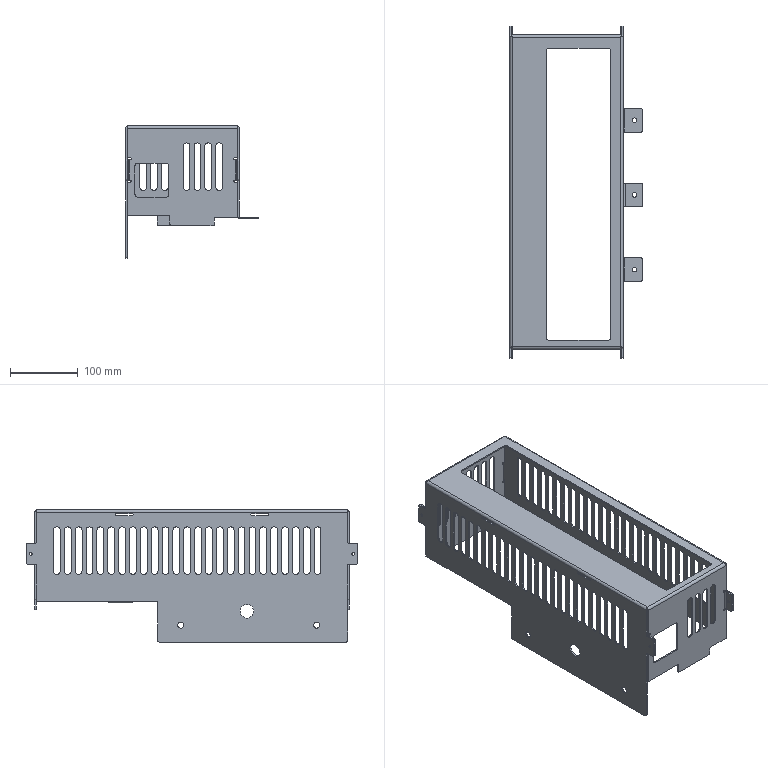Part | STEP file | 68341469 | 1 solid | 534 faces | box 195 x 489 x 195 mm | volume 358150 mm3 | plane 275 | cylinder 245 | spline 14 | commonest cylinder face diameters 10 x125 4 x59 3 x28 8 x14 7 x10 9 x4